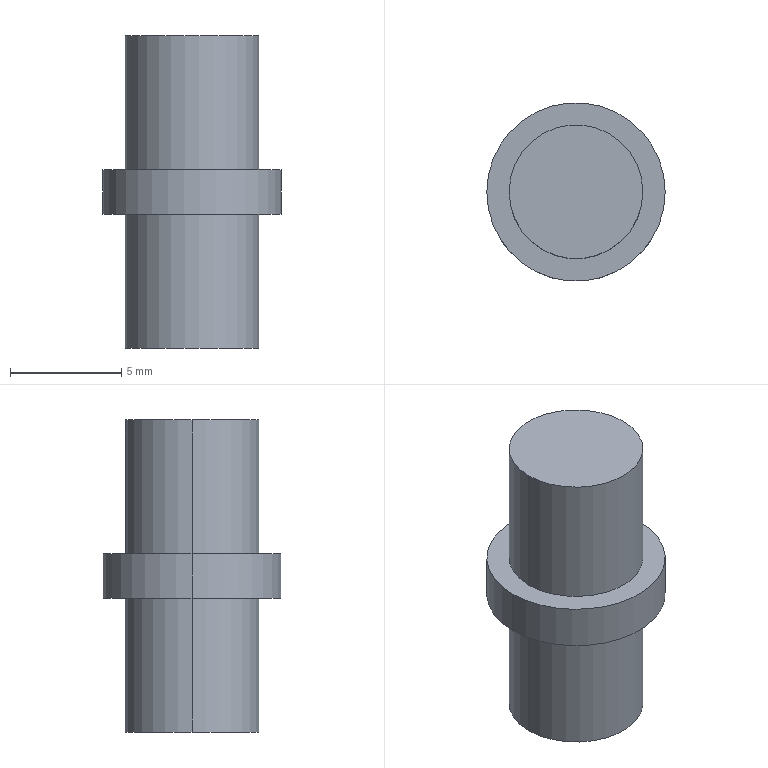Part | STEP file | 001-001-Fixed pin | 1 solid | 10 faces | box 8 x 8 x 14 mm | volume 439.823 mm3 | cylinder 6 | plane 4 | commonest cylinder face diameters 6 x4 8 x2
STEP:
#1=CARTESIAN_POINT('',(0.,0.,0.));
#2=DIRECTION('',(0.,0.,1.));
#3=DIRECTION('',(1.,0.,0.));
#4=AXIS2_PLACEMENT_3D('',#1,#2,#3);
#5=CARTESIAN_POINT('',(798.,-6.5,-6.));
#6=VERTEX_POINT('',#5);
#7=CARTESIAN_POINT('',(792.,-6.5,-6.));
#8=VERTEX_POINT('',#7);
#9=CARTESIAN_POINT('',(795.,-6.5,-6.));
#10=DIRECTION('',(0.,0.,1.));
#11=DIRECTION('',(1.,0.,0.));
#12=AXIS2_PLACEMENT_3D('',#9,#10,#11);
#13=CIRCLE('',#12,3.);
#14=CARTESIAN_POINT('',(795.,-6.5,-6.));
#15=DIRECTION('',(0.,0.,1.));
#16=DIRECTION('',(1.,0.,0.));
#17=AXIS2_PLACEMENT_3D('',#14,#15,#16);
#18=CYLINDRICAL_SURFACE('',#17,3.);
#19=CARTESIAN_POINT('',(0.,0.));
#20=DIRECTION('',(1.,0.));
#21=VECTOR('',#20,1.);
#22=LINE('',#19,#21);
#23=(GEOMETRIC_REPRESENTATION_CONTEXT(2)PARAMETRIC_REPRESENTATION_CONTEXT()REPRESENTATION_CONTEXT('',''));
#24=DEFINITIONAL_REPRESENTATION('',(#22),#23);
#25=PCURVE('',#18,#24);
#26=CARTESIAN_POINT('',(795.,-6.5,-6.));
#27=DIRECTION('',(0.,0.,1.));
#28=DIRECTION('',(1.,0.,0.));
#29=AXIS2_PLACEMENT_3D('',#26,#27,#28);
#30=PLANE('',#29);
#31=CARTESIAN_POINT('',(0.,0.));
#32=DIRECTION('',(1.,0.));
#33=AXIS2_PLACEMENT_2D('',#31,#32);
#34=CIRCLE('',#33,3.);
#35=(GEOMETRIC_REPRESENTATION_CONTEXT(2)PARAMETRIC_REPRESENTATION_CONTEXT()REPRESENTATION_CONTEXT('',''));
#36=DEFINITIONAL_REPRESENTATION('',(#34),#35);
#37=PCURVE('',#30,#36);
#38=SURFACE_CURVE('',#13,(#25,#37),.PCURVE_S1.);
#39=EDGE_CURVE('',#6,#8,#38,.T.);
#40=ORIENTED_EDGE('',*,*,#39,.T.);
#41=CARTESIAN_POINT('',(792.,-6.5,0.));
#42=VERTEX_POINT('',#41);
#43=CARTESIAN_POINT('',(792.,-6.5,-6.));
#44=DIRECTION('',(0.,0.,1.));
#45=VECTOR('',#44,1.);
#46=LINE('',#43,#45);
#47=CARTESIAN_POINT('',(3.142,0.));
#48=DIRECTION('',(0.,1.));
#49=VECTOR('',#48,1.);
#50=LINE('',#47,#49);
#51=(GEOMETRIC_REPRESENTATION_CONTEXT(2)PARAMETRIC_REPRESENTATION_CONTEXT()REPRESENTATION_CONTEXT('',''));
#52=DEFINITIONAL_REPRESENTATION('',(#50),#51);
#53=PCURVE('',#18,#52);
#54=CARTESIAN_POINT('',(795.,-6.5,-6.));
#55=DIRECTION('',(0.,0.,1.));
#56=DIRECTION('',(1.,0.,0.));
#57=AXIS2_PLACEMENT_3D('',#54,#55,#56);
#58=CYLINDRICAL_SURFACE('',#57,3.);
#59=CARTESIAN_POINT('',(3.142,0.));
#60=DIRECTION('',(0.,1.));
#61=VECTOR('',#60,1.);
#62=LINE('',#59,#61);
#63=(GEOMETRIC_REPRESENTATION_CONTEXT(2)PARAMETRIC_REPRESENTATION_CONTEXT()REPRESENTATION_CONTEXT('',''));
#64=DEFINITIONAL_REPRESENTATION('',(#62),#63);
#65=PCURVE('',#58,#64);
#66=SURFACE_CURVE('',#46,(#53,#65),.PCURVE_S1.);
#67=EDGE_CURVE('',#8,#42,#66,.T.);
#68=ORIENTED_EDGE('',*,*,#67,.T.);
#69=CARTESIAN_POINT('',(798.,-6.5,0.));
#70=VERTEX_POINT('',#69);
#71=CARTESIAN_POINT('',(795.,-6.5,0.));
#72=DIRECTION('',(0.,0.,1.));
#73=DIRECTION('',(1.,0.,0.));
#74=AXIS2_PLACEMENT_3D('',#71,#72,#73);
#75=CIRCLE('',#74,3.);
#76=CARTESIAN_POINT('',(0.,6.));
#77=DIRECTION('',(1.,0.));
#78=VECTOR('',#77,1.);
#79=LINE('',#76,#78);
#80=(GEOMETRIC_REPRESENTATION_CONTEXT(2)PARAMETRIC_REPRESENTATION_CONTEXT()REPRESENTATION_CONTEXT('',''));
#81=DEFINITIONAL_REPRESENTATION('',(#79),#80);
#82=PCURVE('',#18,#81);
#83=CARTESIAN_POINT('',(795.,-6.5,0.));
#84=DIRECTION('',(0.,0.,1.));
#85=DIRECTION('',(1.,0.,0.));
#86=AXIS2_PLACEMENT_3D('',#83,#84,#85);
#87=PLANE('',#86);
#88=CARTESIAN_POINT('',(0.,0.));
#89=DIRECTION('',(1.,0.));
#90=AXIS2_PLACEMENT_2D('',#88,#89);
#91=CIRCLE('',#90,3.);
#92=(GEOMETRIC_REPRESENTATION_CONTEXT(2)PARAMETRIC_REPRESENTATION_CONTEXT()REPRESENTATION_CONTEXT('',''));
#93=DEFINITIONAL_REPRESENTATION('',(#91),#92);
#94=PCURVE('',#87,#93);
#95=SURFACE_CURVE('',#75,(#82,#94),.PCURVE_S1.);
#96=EDGE_CURVE('',#70,#42,#95,.T.);
#97=ORIENTED_EDGE('',*,*,#96,.F.);
#98=CARTESIAN_POINT('',(798.,-6.5,-6.));
#99=DIRECTION('',(0.,0.,1.));
#100=VECTOR('',#99,1.);
#101=LINE('',#98,#100);
#102=CARTESIAN_POINT('',(0.,0.));
#103=DIRECTION('',(0.,1.));
#104=VECTOR('',#103,1.);
#105=LINE('',#102,#104);
#106=(GEOMETRIC_REPRESENTATION_CONTEXT(2)PARAMETRIC_REPRESENTATION_CONTEXT()REPRESENTATION_CONTEXT('',''));
#107=DEFINITIONAL_REPRESENTATION('',(#105),#106);
#108=PCURVE('',#18,#107);
#109=CARTESIAN_POINT('',(6.283,0.));
#110=DIRECTION('',(0.,1.));
#111=VECTOR('',#110,1.);
#112=LINE('',#109,#111);
#113=(GEOMETRIC_REPRESENTATION_CONTEXT(2)PARAMETRIC_REPRESENTATION_CONTEXT()REPRESENTATION_CONTEXT('',''));
#114=DEFINITIONAL_REPRESENTATION('',(#112),#113);
#115=PCURVE('',#58,#114);
#116=SURFACE_CURVE('',#101,(#108,#115),.PCURVE_S1.);
#117=EDGE_CURVE('',#6,#70,#116,.T.);
#118=ORIENTED_EDGE('',*,*,#117,.F.);
#119=EDGE_LOOP('',(#40,#68,#97,#118));
#120=FACE_BOUND('',#119,.T.);
#121=ADVANCED_FACE('',(#120),#18,.T.);
#122=CARTESIAN_POINT('',(799.,-6.5,2.));
#123=VERTEX_POINT('',#122);
#124=CARTESIAN_POINT('',(791.,-6.5,2.));
#125=VERTEX_POINT('',#124);
#126=CARTESIAN_POINT('',(795.,-6.5,2.));
#127=DIRECTION('',(0.,0.,1.));
#128=DIRECTION('',(1.,0.,0.));
#129=AXIS2_PLACEMENT_3D('',#126,#127,#128);
#130=CIRCLE('',#129,4.);
#131=CARTESIAN_POINT('',(795.,-6.5,2.));
#132=DIRECTION('',(0.,0.,-1.));
#133=DIRECTION('',(-1.,0.,0.));
#134=AXIS2_PLACEMENT_3D('',#131,#132,#133);
#135=CYLINDRICAL_SURFACE('',#134,4.);
#136=CARTESIAN_POINT('',(3.142,0.));
#137=DIRECTION('',(-1.,0.));
#138=VECTOR('',#137,1.);
#139=LINE('',#136,#138);
#140=(GEOMETRIC_REPRESENTATION_CONTEXT(2)PARAMETRIC_REPRESENTATION_CONTEXT()REPRESENTATION_CONTEXT('',''));
#141=DEFINITIONAL_REPRESENTATION('',(#139),#140);
#142=PCURVE('',#135,#141);
#143=CARTESIAN_POINT('',(795.,-6.5,2.));
#144=DIRECTION('',(0.,0.,1.));
#145=DIRECTION('',(1.,0.,0.));
#146=AXIS2_PLACEMENT_3D('',#143,#144,#145);
#147=PLANE('',#146);
#148=CARTESIAN_POINT('',(0.,0.));
#149=DIRECTION('',(1.,0.));
#150=AXIS2_PLACEMENT_2D('',#148,#149);
#151=CIRCLE('',#150,4.);
#152=(GEOMETRIC_REPRESENTATION_CONTEXT(2)PARAMETRIC_REPRESENTATION_CONTEXT()REPRESENTATION_CONTEXT('',''));
#153=DEFINITIONAL_REPRESENTATION('',(#151),#152);
#154=PCURVE('',#147,#153);
#155=SURFACE_CURVE('',#130,(#142,#154),.PCURVE_S1.);
#156=EDGE_CURVE('',#123,#125,#155,.T.);
#157=ORIENTED_EDGE('',*,*,#156,.F.);
#158=CARTESIAN_POINT('',(799.,-6.5,0.));
#159=VERTEX_POINT('',#158);
#160=CARTESIAN_POINT('',(799.,-6.5,2.));
#161=DIRECTION('',(0.,0.,-1.));
#162=VECTOR('',#161,1.);
#163=LINE('',#160,#162);
#164=CARTESIAN_POINT('',(3.142,0.));
#165=DIRECTION('',(0.,1.));
#166=VECTOR('',#165,1.);
#167=LINE('',#164,#166);
#168=(GEOMETRIC_REPRESENTATION_CONTEXT(2)PARAMETRIC_REPRESENTATION_CONTEXT()REPRESENTATION_CONTEXT('',''));
#169=DEFINITIONAL_REPRESENTATION('',(#167),#168);
#170=PCURVE('',#135,#169);
#171=CARTESIAN_POINT('',(795.,-6.5,2.));
#172=DIRECTION('',(0.,0.,-1.));
#173=DIRECTION('',(-1.,0.,0.));
#174=AXIS2_PLACEMENT_3D('',#171,#172,#173);
#175=CYLINDRICAL_SURFACE('',#174,4.);
#176=CARTESIAN_POINT('',(3.142,0.));
#177=DIRECTION('',(0.,1.));
#178=VECTOR('',#177,1.);
#179=LINE('',#176,#178);
#180=(GEOMETRIC_REPRESENTATION_CONTEXT(2)PARAMETRIC_REPRESENTATION_CONTEXT()REPRESENTATION_CONTEXT('',''));
#181=DEFINITIONAL_REPRESENTATION('',(#179),#180);
#182=PCURVE('',#175,#181);
#183=SURFACE_CURVE('',#163,(#170,#182),.PCURVE_S1.);
#184=EDGE_CURVE('',#123,#159,#183,.T.);
#185=ORIENTED_EDGE('',*,*,#184,.T.);
#186=CARTESIAN_POINT('',(791.,-6.5,0.));
#187=VERTEX_POINT('',#186);
#188=CARTESIAN_POINT('',(795.,-6.5,0.));
#189=DIRECTION('',(0.,0.,1.));
#190=DIRECTION('',(1.,0.,0.));
#191=AXIS2_PLACEMENT_3D('',#188,#189,#190);
#192=CIRCLE('',#191,4.);
#193=CARTESIAN_POINT('',(3.142,2.));
#194=DIRECTION('',(-1.,0.));
#195=VECTOR('',#194,1.);
#196=LINE('',#193,#195);
#197=(GEOMETRIC_REPRESENTATION_CONTEXT(2)PARAMETRIC_REPRESENTATION_CONTEXT()REPRESENTATION_CONTEXT('',''));
#198=DEFINITIONAL_REPRESENTATION('',(#196),#197);
#199=PCURVE('',#135,#198);
#200=CARTESIAN_POINT('',(0.,0.));
#201=DIRECTION('',(1.,0.));
#202=AXIS2_PLACEMENT_2D('',#200,#201);
#203=CIRCLE('',#202,4.);
#204=(GEOMETRIC_REPRESENTATION_CONTEXT(2)PARAMETRIC_REPRESENTATION_CONTEXT()REPRESENTATION_CONTEXT('',''));
#205=DEFINITIONAL_REPRESENTATION('',(#203),#204);
#206=PCURVE('',#87,#205);
#207=SURFACE_CURVE('',#192,(#199,#206),.PCURVE_S1.);
#208=EDGE_CURVE('',#159,#187,#207,.T.);
#209=ORIENTED_EDGE('',*,*,#208,.T.);
#210=CARTESIAN_POINT('',(791.,-6.5,2.));
#211=DIRECTION('',(0.,0.,-1.));
#212=VECTOR('',#211,1.);
#213=LINE('',#210,#212);
#214=CARTESIAN_POINT('',(0.,0.));
#215=DIRECTION('',(0.,1.));
#216=VECTOR('',#215,1.);
#217=LINE('',#214,#216);
#218=(GEOMETRIC_REPRESENTATION_CONTEXT(2)PARAMETRIC_REPRESENTATION_CONTEXT()REPRESENTATION_CONTEXT('',''));
#219=DEFINITIONAL_REPRESENTATION('',(#217),#218);
#220=PCURVE('',#135,#219);
#221=CARTESIAN_POINT('',(6.283,0.));
#222=DIRECTION('',(0.,1.));
#223=VECTOR('',#222,1.);
#224=LINE('',#221,#223);
#225=(GEOMETRIC_REPRESENTATION_CONTEXT(2)PARAMETRIC_REPRESENTATION_CONTEXT()REPRESENTATION_CONTEXT('',''));
#226=DEFINITIONAL_REPRESENTATION('',(#224),#225);
#227=PCURVE('',#175,#226);
#228=SURFACE_CURVE('',#213,(#220,#227),.PCURVE_S1.);
#229=EDGE_CURVE('',#125,#187,#228,.T.);
#230=ORIENTED_EDGE('',*,*,#229,.F.);
#231=EDGE_LOOP('',(#157,#185,#209,#230));
#232=FACE_BOUND('',#231,.T.);
#233=ADVANCED_FACE('',(#232),#135,.T.);
#234=CARTESIAN_POINT('',(792.,-6.5,2.));
#235=VERTEX_POINT('',#234);
#236=CARTESIAN_POINT('',(798.,-6.5,2.));
#237=VERTEX_POINT('',#236);
#238=CARTESIAN_POINT('',(795.,-6.5,2.));
#239=DIRECTION('',(0.,0.,-1.));
#240=DIRECTION('',(1.,0.,0.));
#241=AXIS2_PLACEMENT_3D('',#238,#239,#240);
#242=CIRCLE('',#241,3.);
#243=CARTESIAN_POINT('',(795.,-6.5,-6.));
#244=DIRECTION('',(0.,0.,1.));
#245=DIRECTION('',(1.,0.,0.));
#246=AXIS2_PLACEMENT_3D('',#243,#244,#245);
#247=CYLINDRICAL_SURFACE('',#246,3.);
#248=CARTESIAN_POINT('',(6.283,8.));
#249=DIRECTION('',(-1.,0.));
#250=VECTOR('',#249,1.);
#251=LINE('',#248,#250);
#252=(GEOMETRIC_REPRESENTATION_CONTEXT(2)PARAMETRIC_REPRESENTATION_CONTEXT()REPRESENTATION_CONTEXT('',''));
#253=DEFINITIONAL_REPRESENTATION('',(#251),#252);
#254=PCURVE('',#247,#253);
#255=CARTESIAN_POINT('',(3.,0.));
#256=CARTESIAN_POINT('',(3.,-5.196));
#257=CARTESIAN_POINT('',(-1.5,-2.598));
#258=CARTESIAN_POINT('',(-6.,0.));
#259=CARTESIAN_POINT('',(-1.5,2.598));
#260=CARTESIAN_POINT('',(3.,5.196));
#261=CARTESIAN_POINT('',(3.,0.));
#262=(BOUNDED_CURVE()B_SPLINE_CURVE(2,(#255,#256,#257,#258,#259,#260,#261),.UNSPECIFIED.,.T.,.F.)B_SPLINE_CURVE_WITH_KNOTS((1,2,2,2,2,1),(-2.094,0.,2.094,4.189,6.283,8.378),.UNSPECIFIED.)CURVE()GEOMETRIC_REPRESENTATION_ITEM()RATIONAL_B_SPLINE_CURVE((1.,0.5,1.,0.5,1.,0.5,1.))REPRESENTATION_ITEM(''));
#263=(GEOMETRIC_REPRESENTATION_CONTEXT(2)PARAMETRIC_REPRESENTATION_CONTEXT()REPRESENTATION_CONTEXT('',''));
#264=DEFINITIONAL_REPRESENTATION('',(#262),#263);
#265=PCURVE('',#147,#264);
#266=SURFACE_CURVE('',#242,(#254,#265),.PCURVE_S1.);
#267=EDGE_CURVE('',#235,#237,#266,.T.);
#268=ORIENTED_EDGE('',*,*,#267,.F.);
#269=CARTESIAN_POINT('',(792.,-6.5,8.));
#270=VERTEX_POINT('',#269);
#271=CARTESIAN_POINT('',(792.,-6.5,-6.));
#272=DIRECTION('',(0.,0.,1.));
#273=VECTOR('',#272,1.);
#274=LINE('',#271,#273);
#275=CARTESIAN_POINT('',(3.142,0.));
#276=DIRECTION('',(0.,1.));
#277=VECTOR('',#276,1.);
#278=LINE('',#275,#277);
#279=(GEOMETRIC_REPRESENTATION_CONTEXT(2)PARAMETRIC_REPRESENTATION_CONTEXT()REPRESENTATION_CONTEXT('',''));
#280=DEFINITIONAL_REPRESENTATION('',(#278),#279);
#281=PCURVE('',#247,#280);
#282=CARTESIAN_POINT('',(795.,-6.5,-6.));
#283=DIRECTION('',(0.,0.,1.));
#284=DIRECTION('',(1.,0.,0.));
#285=AXIS2_PLACEMENT_3D('',#282,#283,#284);
#286=CYLINDRICAL_SURFACE('',#285,3.);
#287=CARTESIAN_POINT('',(3.142,0.));
#288=DIRECTION('',(0.,1.));
#289=VECTOR('',#288,1.);
#290=LINE('',#287,#289);
#291=(GEOMETRIC_REPRESENTATION_CONTEXT(2)PARAMETRIC_REPRESENTATION_CONTEXT()REPRESENTATION_CONTEXT('',''));
#292=DEFINITIONAL_REPRESENTATION('',(#290),#291);
#293=PCURVE('',#286,#292);
#294=SURFACE_CURVE('',#274,(#281,#293),.PCURVE_S1.);
#295=EDGE_CURVE('',#235,#270,#294,.T.);
#296=ORIENTED_EDGE('',*,*,#295,.T.);
#297=CARTESIAN_POINT('',(798.,-6.5,8.));
#298=VERTEX_POINT('',#297);
#299=CARTESIAN_POINT('',(795.,-6.5,8.));
#300=DIRECTION('',(0.,0.,1.));
#301=DIRECTION('',(1.,0.,0.));
#302=AXIS2_PLACEMENT_3D('',#299,#300,#301);
#303=CIRCLE('',#302,3.);
#304=CARTESIAN_POINT('',(0.,14.));
#305=DIRECTION('',(1.,0.));
#306=VECTOR('',#305,1.);
#307=LINE('',#304,#306);
#308=(GEOMETRIC_REPRESENTATION_CONTEXT(2)PARAMETRIC_REPRESENTATION_CONTEXT()REPRESENTATION_CONTEXT('',''));
#309=DEFINITIONAL_REPRESENTATION('',(#307),#308);
#310=PCURVE('',#247,#309);
#311=CARTESIAN_POINT('',(795.,-6.5,8.));
#312=DIRECTION('',(0.,0.,1.));
#313=DIRECTION('',(1.,0.,0.));
#314=AXIS2_PLACEMENT_3D('',#311,#312,#313);
#315=PLANE('',#314);
#316=CARTESIAN_POINT('',(0.,0.));
#317=DIRECTION('',(1.,0.));
#318=AXIS2_PLACEMENT_2D('',#316,#317);
#319=CIRCLE('',#318,3.);
#320=(GEOMETRIC_REPRESENTATION_CONTEXT(2)PARAMETRIC_REPRESENTATION_CONTEXT()REPRESENTATION_CONTEXT('',''));
#321=DEFINITIONAL_REPRESENTATION('',(#319),#320);
#322=PCURVE('',#315,#321);
#323=SURFACE_CURVE('',#303,(#310,#322),.PCURVE_S1.);
#324=EDGE_CURVE('',#298,#270,#323,.T.);
#325=ORIENTED_EDGE('',*,*,#324,.F.);
#326=CARTESIAN_POINT('',(798.,-6.5,-6.));
#327=DIRECTION('',(0.,0.,1.));
#328=VECTOR('',#327,1.);
#329=LINE('',#326,#328);
#330=CARTESIAN_POINT('',(0.,0.));
#331=DIRECTION('',(0.,1.));
#332=VECTOR('',#331,1.);
#333=LINE('',#330,#332);
#334=(GEOMETRIC_REPRESENTATION_CONTEXT(2)PARAMETRIC_REPRESENTATION_CONTEXT()REPRESENTATION_CONTEXT('',''));
#335=DEFINITIONAL_REPRESENTATION('',(#333),#334);
#336=PCURVE('',#247,#335);
#337=CARTESIAN_POINT('',(6.283,0.));
#338=DIRECTION('',(0.,1.));
#339=VECTOR('',#338,1.);
#340=LINE('',#337,#339);
#341=(GEOMETRIC_REPRESENTATION_CONTEXT(2)PARAMETRIC_REPRESENTATION_CONTEXT()REPRESENTATION_CONTEXT('',''));
#342=DEFINITIONAL_REPRESENTATION('',(#340),#341);
#343=PCURVE('',#286,#342);
#344=SURFACE_CURVE('',#329,(#336,#343),.PCURVE_S1.);
#345=EDGE_CURVE('',#237,#298,#344,.T.);
#346=ORIENTED_EDGE('',*,*,#345,.F.);
#347=EDGE_LOOP('',(#268,#296,#325,#346));
#348=FACE_BOUND('',#347,.T.);
#349=ADVANCED_FACE('',(#348),#247,.T.);
#350=ORIENTED_EDGE('',*,*,#295,.F.);
#351=CARTESIAN_POINT('',(795.,-6.5,2.));
#352=DIRECTION('',(0.,0.,-1.));
#353=DIRECTION('',(1.,0.,0.));
#354=AXIS2_PLACEMENT_3D('',#351,#352,#353);
#355=CIRCLE('',#354,3.);
#356=CARTESIAN_POINT('',(6.283,8.));
#357=DIRECTION('',(-1.,0.));
#358=VECTOR('',#357,1.);
#359=LINE('',#356,#358);
#360=(GEOMETRIC_REPRESENTATION_CONTEXT(2)PARAMETRIC_REPRESENTATION_CONTEXT()REPRESENTATION_CONTEXT('',''));
#361=DEFINITIONAL_REPRESENTATION('',(#359),#360);
#362=PCURVE('',#286,#361);
#363=CARTESIAN_POINT('',(3.,0.));
#364=CARTESIAN_POINT('',(3.,-5.196));
#365=CARTESIAN_POINT('',(-1.5,-2.598));
#366=CARTESIAN_POINT('',(-6.,0.));
#367=CARTESIAN_POINT('',(-1.5,2.598));
#368=CARTESIAN_POINT('',(3.,5.196));
#369=CARTESIAN_POINT('',(3.,0.));
#370=(BOUNDED_CURVE()B_SPLINE_CURVE(2,(#363,#364,#365,#366,#367,#368,#369),.UNSPECIFIED.,.T.,.F.)B_SPLINE_CURVE_WITH_KNOTS((1,2,2,2,2,1),(-2.094,0.,2.094,4.189,6.283,8.378),.UNSPECIFIED.)CURVE()GEOMETRIC_REPRESENTATION_ITEM()RATIONAL_B_SPLINE_CURVE((1.,0.5,1.,0.5,1.,0.5,1.))REPRESENTATION_ITEM(''));
#371=(GEOMETRIC_REPRESENTATION_CONTEXT(2)PARAMETRIC_REPRESENTATION_CONTEXT()REPRESENTATION_CONTEXT('',''));
#372=DEFINITIONAL_REPRESENTATION('',(#370),#371);
#373=PCURVE('',#147,#372);
#374=SURFACE_CURVE('',#355,(#362,#373),.PCURVE_S1.);
#375=EDGE_CURVE('',#237,#235,#374,.T.);
#376=ORIENTED_EDGE('',*,*,#375,.F.);
#377=ORIENTED_EDGE('',*,*,#345,.T.);
#378=CARTESIAN_POINT('',(795.,-6.5,8.));
#379=DIRECTION('',(0.,0.,1.));
#380=DIRECTION('',(1.,0.,0.));
#381=AXIS2_PLACEMENT_3D('',#378,#379,#380);
#382=CIRCLE('',#381,3.);
#383=CARTESIAN_POINT('',(0.,14.));
#384=DIRECTION('',(1.,0.));
#385=VECTOR('',#384,1.);
#386=LINE('',#383,#385);
#387=(GEOMETRIC_REPRESENTATION_CONTEXT(2)PARAMETRIC_REPRESENTATION_CONTEXT()REPRESENTATION_CONTEXT('',''));
#388=DEFINITIONAL_REPRESENTATION('',(#386),#387);
#389=PCURVE('',#286,#388);
#390=CARTESIAN_POINT('',(0.,0.));
#391=DIRECTION('',(1.,0.));
#392=AXIS2_PLACEMENT_2D('',#390,#391);
#393=CIRCLE('',#392,3.);
#394=(GEOMETRIC_REPRESENTATION_CONTEXT(2)PARAMETRIC_REPRESENTATION_CONTEXT()REPRESENTATION_CONTEXT('',''));
#395=DEFINITIONAL_REPRESENTATION('',(#393),#394);
#396=PCURVE('',#315,#395);
#397=SURFACE_CURVE('',#382,(#389,#396),.PCURVE_S1.);
#398=EDGE_CURVE('',#270,#298,#397,.T.);
#399=ORIENTED_EDGE('',*,*,#398,.F.);
#400=EDGE_LOOP('',(#350,#376,#377,#399));
#401=FACE_BOUND('',#400,.T.);
#402=ADVANCED_FACE('',(#401),#286,.T.);
#403=ORIENTED_EDGE('',*,*,#324,.T.);
#404=ORIENTED_EDGE('',*,*,#398,.T.);
#405=EDGE_LOOP('',(#403,#404));
#406=FACE_BOUND('',#405,.T.);
#407=ADVANCED_FACE('',(#406),#315,.T.);
#408=CARTESIAN_POINT('',(795.,-6.5,2.));
#409=DIRECTION('',(0.,0.,1.));
#410=DIRECTION('',(1.,0.,0.));
#411=AXIS2_PLACEMENT_3D('',#408,#409,#410);
#412=CIRCLE('',#411,4.);
#413=CARTESIAN_POINT('',(0.,0.));
#414=DIRECTION('',(1.,0.));
#415=AXIS2_PLACEMENT_2D('',#413,#414);
#416=CIRCLE('',#415,4.);
#417=(GEOMETRIC_REPRESENTATION_CONTEXT(2)PARAMETRIC_REPRESENTATION_CONTEXT()REPRESENTATION_CONTEXT('',''));
#418=DEFINITIONAL_REPRESENTATION('',(#416),#417);
#419=PCURVE('',#147,#418);
#420=CARTESIAN_POINT('',(9.425,0.));
#421=DIRECTION('',(-1.,0.));
#422=VECTOR('',#421,1.);
#423=LINE('',#420,#422);
#424=(GEOMETRIC_REPRESENTATION_CONTEXT(2)PARAMETRIC_REPRESENTATION_CONTEXT()REPRESENTATION_CONTEXT('',''));
#425=DEFINITIONAL_REPRESENTATION('',(#423),#424);
#426=PCURVE('',#175,#425);
#427=SURFACE_CURVE('',#412,(#419,#426),.PCURVE_S1.);
#428=EDGE_CURVE('',#125,#123,#427,.T.);
#429=ORIENTED_EDGE('',*,*,#428,.T.);
#430=ORIENTED_EDGE('',*,*,#156,.T.);
#431=EDGE_LOOP('',(#429,#430));
#432=FACE_BOUND('',#431,.T.);
#433=ORIENTED_EDGE('',*,*,#375,.T.);
#434=ORIENTED_EDGE('',*,*,#267,.T.);
#435=EDGE_LOOP('',(#433,#434));
#436=FACE_BOUND('',#435,.T.);
#437=ADVANCED_FACE('',(#432,#436),#147,.T.);
#438=CARTESIAN_POINT('',(795.,-6.5,0.));
#439=DIRECTION('',(0.,0.,1.));
#440=DIRECTION('',(1.,0.,0.));
#441=AXIS2_PLACEMENT_3D('',#438,#439,#440);
#442=CIRCLE('',#441,4.);
#443=CARTESIAN_POINT('',(0.,0.));
#444=DIRECTION('',(1.,0.));
#445=AXIS2_PLACEMENT_2D('',#443,#444);
#446=CIRCLE('',#445,4.);
#447=(GEOMETRIC_REPRESENTATION_CONTEXT(2)PARAMETRIC_REPRESENTATION_CONTEXT()REPRESENTATION_CONTEXT('',''));
#448=DEFINITIONAL_REPRESENTATION('',(#446),#447);
#449=PCURVE('',#87,#448);
#450=CARTESIAN_POINT('',(9.425,2.));
#451=DIRECTION('',(-1.,0.));
#452=VECTOR('',#451,1.);
#453=LINE('',#450,#452);
#454=(GEOMETRIC_REPRESENTATION_CONTEXT(2)PARAMETRIC_REPRESENTATION_CONTEXT()REPRESENTATION_CONTEXT('',''));
#455=DEFINITIONAL_REPRESENTATION('',(#453),#454);
#456=PCURVE('',#175,#455);
#457=SURFACE_CURVE('',#442,(#449,#456),.PCURVE_S1.);
#458=EDGE_CURVE('',#187,#159,#457,.T.);
#459=ORIENTED_EDGE('',*,*,#458,.F.);
#460=ORIENTED_EDGE('',*,*,#208,.F.);
#461=EDGE_LOOP('',(#459,#460));
#462=FACE_BOUND('',#461,.T.);
#463=ORIENTED_EDGE('',*,*,#96,.T.);
#464=CARTESIAN_POINT('',(795.,-6.5,0.));
#465=DIRECTION('',(0.,0.,1.));
#466=DIRECTION('',(1.,0.,0.));
#467=AXIS2_PLACEMENT_3D('',#464,#465,#466);
#468=CIRCLE('',#467,3.);
#469=CARTESIAN_POINT('',(0.,0.));
#470=DIRECTION('',(1.,0.));
#471=AXIS2_PLACEMENT_2D('',#469,#470);
#472=CIRCLE('',#471,3.);
#473=(GEOMETRIC_REPRESENTATION_CONTEXT(2)PARAMETRIC_REPRESENTATION_CONTEXT()REPRESENTATION_CONTEXT('',''));
#474=DEFINITIONAL_REPRESENTATION('',(#472),#473);
#475=PCURVE('',#87,#474);
#476=CARTESIAN_POINT('',(0.,6.));
#477=DIRECTION('',(1.,0.));
#478=VECTOR('',#477,1.);
#479=LINE('',#476,#478);
#480=(GEOMETRIC_REPRESENTATION_CONTEXT(2)PARAMETRIC_REPRESENTATION_CONTEXT()REPRESENTATION_CONTEXT('',''));
#481=DEFINITIONAL_REPRESENTATION('',(#479),#480);
#482=PCURVE('',#58,#481);
#483=SURFACE_CURVE('',#468,(#475,#482),.PCURVE_S1.);
#484=EDGE_CURVE('',#42,#70,#483,.T.);
#485=ORIENTED_EDGE('',*,*,#484,.T.);
#486=EDGE_LOOP('',(#463,#485));
#487=FACE_BOUND('',#486,.T.);
#488=ADVANCED_FACE('',(#462,#487),#87,.F.);
#489=ORIENTED_EDGE('',*,*,#184,.F.);
#490=ORIENTED_EDGE('',*,*,#428,.F.);
#491=ORIENTED_EDGE('',*,*,#229,.T.);
#492=ORIENTED_EDGE('',*,*,#458,.T.);
#493=EDGE_LOOP('',(#489,#490,#491,#492));
#494=FACE_BOUND('',#493,.T.);
#495=ADVANCED_FACE('',(#494),#175,.T.);
#496=ORIENTED_EDGE('',*,*,#39,.F.);
#497=CARTESIAN_POINT('',(795.,-6.5,-6.));
#498=DIRECTION('',(0.,0.,1.));
#499=DIRECTION('',(1.,0.,0.));
#500=AXIS2_PLACEMENT_3D('',#497,#498,#499);
#501=CIRCLE('',#500,3.);
#502=CARTESIAN_POINT('',(0.,0.));
#503=DIRECTION('',(1.,0.));
#504=AXIS2_PLACEMENT_2D('',#502,#503);
#505=CIRCLE('',#504,3.);
#506=(GEOMETRIC_REPRESENTATION_CONTEXT(2)PARAMETRIC_REPRESENTATION_CONTEXT()REPRESENTATION_CONTEXT('',''));
#507=DEFINITIONAL_REPRESENTATION('',(#505),#506);
#508=PCURVE('',#30,#507);
#509=CARTESIAN_POINT('',(0.,0.));
#510=DIRECTION('',(1.,0.));
#511=VECTOR('',#510,1.);
#512=LINE('',#509,#511);
#513=(GEOMETRIC_REPRESENTATION_CONTEXT(2)PARAMETRIC_REPRESENTATION_CONTEXT()REPRESENTATION_CONTEXT('',''));
#514=DEFINITIONAL_REPRESENTATION('',(#512),#513);
#515=PCURVE('',#58,#514);
#516=SURFACE_CURVE('',#501,(#508,#515),.PCURVE_S1.);
#517=EDGE_CURVE('',#8,#6,#516,.T.);
#518=ORIENTED_EDGE('',*,*,#517,.F.);
#519=EDGE_LOOP('',(#496,#518));
#520=FACE_BOUND('',#519,.T.);
#521=ADVANCED_FACE('',(#520),#30,.F.);
#522=ORIENTED_EDGE('',*,*,#67,.F.);
#523=ORIENTED_EDGE('',*,*,#517,.T.);
#524=ORIENTED_EDGE('',*,*,#117,.T.);
#525=ORIENTED_EDGE('',*,*,#484,.F.);
#526=EDGE_LOOP('',(#522,#523,#524,#525));
#527=FACE_BOUND('',#526,.T.);
#528=ADVANCED_FACE('',(#527),#58,.T.);
#529=CLOSED_SHELL('',(#121,#233,#349,#402,#407,#437,#488,#495,#521,#528));
#530=MANIFOLD_SOLID_BREP('',#529);
#531=(LENGTH_UNIT()NAMED_UNIT(*)SI_UNIT(.MILLI.,.METRE.));
#532=UNCERTAINTY_MEASURE_WITH_UNIT(LENGTH_MEASURE(0.0000001),#531,'','');
#533=(NAMED_UNIT(*)PLANE_ANGLE_UNIT()SI_UNIT($,.RADIAN.));
#534=(NAMED_UNIT(*)SI_UNIT($,.STERADIAN.)SOLID_ANGLE_UNIT());
#535=(GEOMETRIC_REPRESENTATION_CONTEXT(3)GLOBAL_UNCERTAINTY_ASSIGNED_CONTEXT((#532))GLOBAL_UNIT_ASSIGNED_CONTEXT((#531,#533,#534))REPRESENTATION_CONTEXT('',''));
#536=ADVANCED_BREP_SHAPE_REPRESENTATION('',(#4,#530),#535);